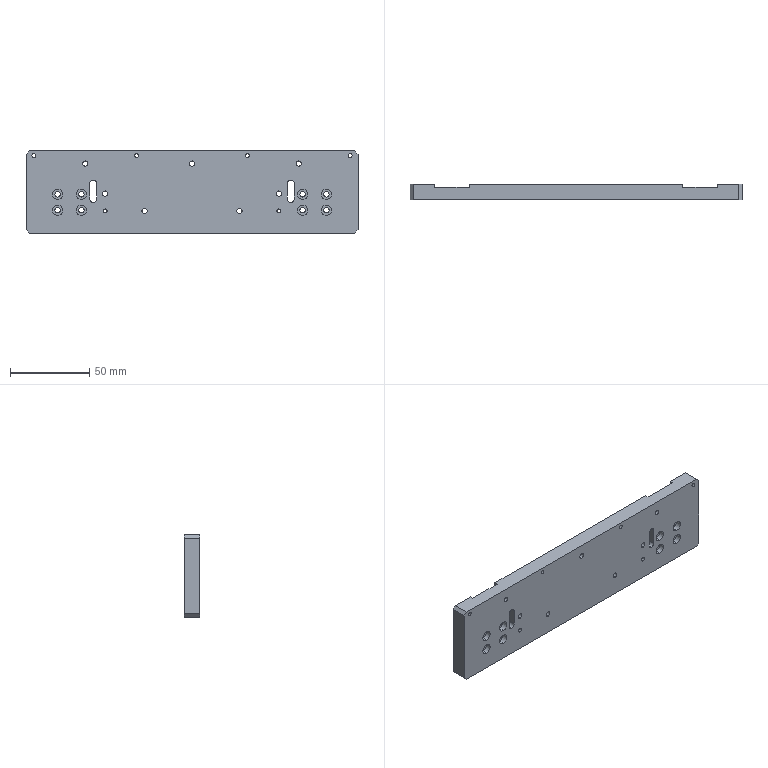Part | STEP file | lift adapter plate 2 | 1 solid | 112 faces | box 210 x 10 x 52 mm | volume 101060 mm3 | cylinder 72 | plane 32 | cone 8 | commonest cylinder face diameters 3.3 x22 3.4 x16 6.5 x16 2.5 x12 4.2 x6